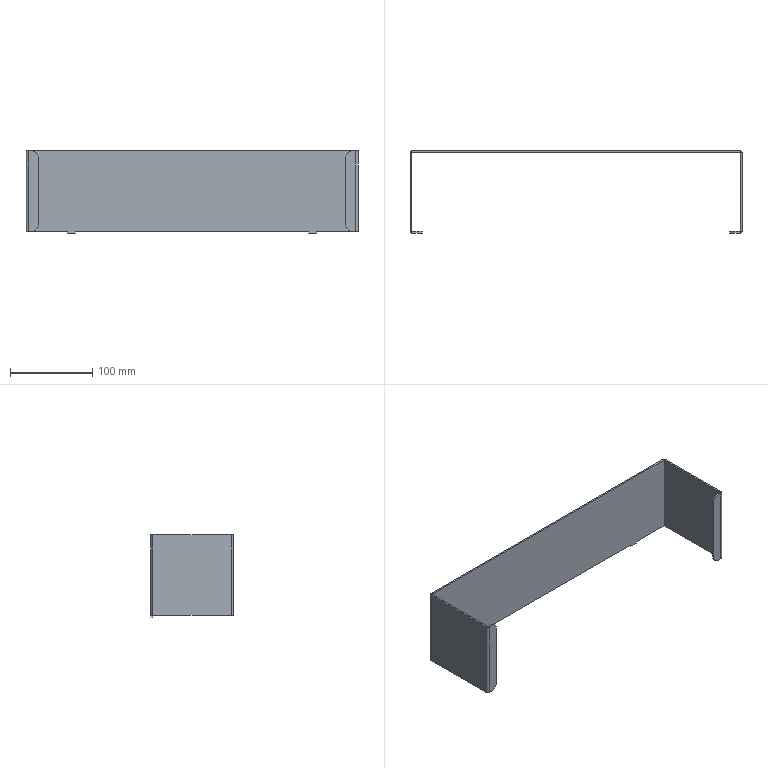Part | STEP file | xzz-001 | 1 solid | 34 faces | box 404 x 100 x 100 mm | volume 122161 mm3 | plane 22 | cylinder 12 | commonest cylinder face diameters 1 x4 5 x4 16 x4
STEP:
#1=CARTESIAN_POINT('',(165.,30.,-2.));
#2=VERTEX_POINT('',#1);
#3=CARTESIAN_POINT('',(175.,30.,-2.));
#4=VERTEX_POINT('',#3);
#5=CARTESIAN_POINT('',(-179.,30.,-2.));
#6=DIRECTION('',(1.,0.,0.));
#7=VECTOR('',#6,1000.);
#8=LINE('',#5,#7);
#9=EDGE_CURVE('',#2,#4,#8,.T.);
#10=ORIENTED_EDGE('',*,*,#9,.T.);
#11=CARTESIAN_POINT('',(175.,30.,0.));
#12=VERTEX_POINT('',#11);
#13=CARTESIAN_POINT('',(175.,30.,98.));
#14=DIRECTION('',(0.,0.,1.));
#15=VECTOR('',#14,1000.);
#16=LINE('',#13,#15);
#17=EDGE_CURVE('',#4,#12,#16,.T.);
#18=ORIENTED_EDGE('',*,*,#17,.T.);
#19=CARTESIAN_POINT('',(222.5,30.,0.));
#20=VERTEX_POINT('',#19);
#21=CARTESIAN_POINT('',(-179.,30.,0.));
#22=DIRECTION('',(1.,0.,0.));
#23=VECTOR('',#22,1000.);
#24=LINE('',#21,#23);
#25=EDGE_CURVE('',#12,#20,#24,.T.);
#26=ORIENTED_EDGE('',*,*,#25,.T.);
#27=CARTESIAN_POINT('',(222.5,30.,98.));
#28=VERTEX_POINT('',#27);
#29=CARTESIAN_POINT('',(222.5,30.,98.));
#30=DIRECTION('',(0.,0.,1.));
#31=VECTOR('',#30,1000.);
#32=LINE('',#29,#31);
#33=EDGE_CURVE('',#20,#28,#32,.T.);
#34=ORIENTED_EDGE('',*,*,#33,.T.);
#35=CARTESIAN_POINT('',(-176.5,30.,98.));
#36=VERTEX_POINT('',#35);
#37=CARTESIAN_POINT('',(-179.,30.,98.));
#38=DIRECTION('',(-1.,0.,0.));
#39=VECTOR('',#38,1000.);
#40=LINE('',#37,#39);
#41=EDGE_CURVE('',#28,#36,#40,.T.);
#42=ORIENTED_EDGE('',*,*,#41,.T.);
#43=CARTESIAN_POINT('',(-176.5,30.,0.));
#44=VERTEX_POINT('',#43);
#45=CARTESIAN_POINT('',(-176.5,30.,98.));
#46=DIRECTION('',(0.,0.,-1.));
#47=VECTOR('',#46,1000.);
#48=LINE('',#45,#47);
#49=EDGE_CURVE('',#36,#44,#48,.T.);
#50=ORIENTED_EDGE('',*,*,#49,.T.);
#51=CARTESIAN_POINT('',(-129.,30.,0.));
#52=VERTEX_POINT('',#51);
#53=CARTESIAN_POINT('',(-179.,30.,0.));
#54=DIRECTION('',(1.,0.,0.));
#55=VECTOR('',#54,1000.);
#56=LINE('',#53,#55);
#57=EDGE_CURVE('',#44,#52,#56,.T.);
#58=ORIENTED_EDGE('',*,*,#57,.T.);
#59=CARTESIAN_POINT('',(-129.,30.,-2.));
#60=VERTEX_POINT('',#59);
#61=CARTESIAN_POINT('',(-129.,30.,98.));
#62=DIRECTION('',(0.,0.,-1.));
#63=VECTOR('',#62,1000.);
#64=LINE('',#61,#63);
#65=EDGE_CURVE('',#52,#60,#64,.T.);
#66=ORIENTED_EDGE('',*,*,#65,.T.);
#67=CARTESIAN_POINT('',(-119.,30.,-2.));
#68=VERTEX_POINT('',#67);
#69=CARTESIAN_POINT('',(-179.,30.,-2.));
#70=DIRECTION('',(1.,0.,0.));
#71=VECTOR('',#70,1000.);
#72=LINE('',#69,#71);
#73=EDGE_CURVE('',#60,#68,#72,.T.);
#74=ORIENTED_EDGE('',*,*,#73,.T.);
#75=CARTESIAN_POINT('',(-119.,30.,0.));
#76=VERTEX_POINT('',#75);
#77=CARTESIAN_POINT('',(-119.,30.,98.));
#78=DIRECTION('',(0.,0.,1.));
#79=VECTOR('',#78,1000.);
#80=LINE('',#77,#79);
#81=EDGE_CURVE('',#68,#76,#80,.T.);
#82=ORIENTED_EDGE('',*,*,#81,.T.);
#83=CARTESIAN_POINT('',(165.,30.,0.));
#84=VERTEX_POINT('',#83);
#85=CARTESIAN_POINT('',(-179.,30.,0.));
#86=DIRECTION('',(1.,0.,0.));
#87=VECTOR('',#86,1000.);
#88=LINE('',#85,#87);
#89=EDGE_CURVE('',#76,#84,#88,.T.);
#90=ORIENTED_EDGE('',*,*,#89,.T.);
#91=CARTESIAN_POINT('',(165.,30.,98.));
#92=DIRECTION('',(0.,0.,-1.));
#93=VECTOR('',#92,1000.);
#94=LINE('',#91,#93);
#95=EDGE_CURVE('',#84,#2,#94,.T.);
#96=ORIENTED_EDGE('',*,*,#95,.T.);
#97=EDGE_LOOP('',(#10,#18,#26,#34,#42,#50,#58,#66,#74,#82,#90,#96));
#98=FACE_OUTER_BOUND('',#97,.T.);
#99=CARTESIAN_POINT('',(-179.,30.,98.));
#100=DIRECTION('',(0.,-1.,0.));
#101=DIRECTION('',(0.,0.,-1.));
#102=AXIS2_PLACEMENT_3D('',#99,#100,#101);
#103=PLANE('',#102);
#104=ADVANCED_FACE('',(#98),#103,.T.);
#105=ORIENTED_EDGE('',*,*,#17,.F.);
#106=CARTESIAN_POINT('',(175.,32.,-2.));
#107=VERTEX_POINT('',#106);
#108=CARTESIAN_POINT('',(175.,32.,-2.));
#109=DIRECTION('',(0.,-1.,0.));
#110=VECTOR('',#109,1000.);
#111=LINE('',#108,#110);
#112=EDGE_CURVE('',#107,#4,#111,.T.);
#113=ORIENTED_EDGE('',*,*,#112,.F.);
#114=CARTESIAN_POINT('',(175.,32.,0.));
#115=VERTEX_POINT('',#114);
#116=CARTESIAN_POINT('',(175.,32.,-2.));
#117=DIRECTION('',(0.,0.,-1.));
#118=VECTOR('',#117,1000.);
#119=LINE('',#116,#118);
#120=EDGE_CURVE('',#115,#107,#119,.T.);
#121=ORIENTED_EDGE('',*,*,#120,.F.);
#122=CARTESIAN_POINT('',(175.,32.,0.));
#123=DIRECTION('',(0.,1.,0.));
#124=VECTOR('',#123,1000.);
#125=LINE('',#122,#124);
#126=EDGE_CURVE('',#12,#115,#125,.T.);
#127=ORIENTED_EDGE('',*,*,#126,.F.);
#128=EDGE_LOOP('',(#105,#113,#121,#127));
#129=FACE_OUTER_BOUND('',#128,.T.);
#130=CARTESIAN_POINT('',(175.,32.,-2.));
#131=DIRECTION('',(-1.,0.,0.));
#132=DIRECTION('',(0.,0.,1.));
#133=AXIS2_PLACEMENT_3D('',#130,#131,#132);
#134=PLANE('',#133);
#135=ADVANCED_FACE('',(#129),#134,.F.);
#136=CARTESIAN_POINT('',(165.,32.,-2.));
#137=VERTEX_POINT('',#136);
#138=CARTESIAN_POINT('',(165.,0.,-2.));
#139=DIRECTION('',(0.,1.,0.));
#140=VECTOR('',#139,1000.);
#141=LINE('',#138,#140);
#142=EDGE_CURVE('',#2,#137,#141,.T.);
#143=ORIENTED_EDGE('',*,*,#142,.T.);
#144=CARTESIAN_POINT('',(0.,32.,-2.));
#145=DIRECTION('',(1.,0.,0.));
#146=VECTOR('',#145,1000.);
#147=LINE('',#144,#146);
#148=EDGE_CURVE('',#137,#107,#147,.T.);
#149=ORIENTED_EDGE('',*,*,#148,.T.);
#150=ORIENTED_EDGE('',*,*,#112,.T.);
#151=ORIENTED_EDGE('',*,*,#9,.F.);
#152=EDGE_LOOP('',(#143,#149,#150,#151));
#153=FACE_OUTER_BOUND('',#152,.T.);
#154=CARTESIAN_POINT('',(0.,0.,-2.));
#155=DIRECTION('',(0.,0.,-1.));
#156=DIRECTION('',(-1.,0.,0.));
#157=AXIS2_PLACEMENT_3D('',#154,#155,#156);
#158=PLANE('',#157);
#159=ADVANCED_FACE('',(#153),#158,.T.);
#160=CARTESIAN_POINT('',(165.,32.,0.));
#161=VERTEX_POINT('',#160);
#162=CARTESIAN_POINT('',(165.,32.,-2.));
#163=DIRECTION('',(0.,0.,1.));
#164=VECTOR('',#163,1000.);
#165=LINE('',#162,#164);
#166=EDGE_CURVE('',#137,#161,#165,.T.);
#167=ORIENTED_EDGE('',*,*,#166,.F.);
#168=ORIENTED_EDGE('',*,*,#142,.F.);
#169=ORIENTED_EDGE('',*,*,#95,.F.);
#170=CARTESIAN_POINT('',(165.,32.,0.));
#171=DIRECTION('',(0.,-1.,0.));
#172=VECTOR('',#171,1000.);
#173=LINE('',#170,#172);
#174=EDGE_CURVE('',#161,#84,#173,.T.);
#175=ORIENTED_EDGE('',*,*,#174,.F.);
#176=EDGE_LOOP('',(#167,#168,#169,#175));
#177=FACE_OUTER_BOUND('',#176,.T.);
#178=CARTESIAN_POINT('',(165.,32.,-2.));
#179=DIRECTION('',(1.,0.,0.));
#180=DIRECTION('',(0.,0.,-1.));
#181=AXIS2_PLACEMENT_3D('',#178,#179,#180);
#182=PLANE('',#181);
#183=ADVANCED_FACE('',(#177),#182,.F.);
#184=CARTESIAN_POINT('',(-119.,32.,0.));
#185=VERTEX_POINT('',#184);
#186=CARTESIAN_POINT('',(223.,32.,0.));
#187=DIRECTION('',(1.,0.,0.));
#188=VECTOR('',#187,1000.);
#189=LINE('',#186,#188);
#190=EDGE_CURVE('',#185,#161,#189,.T.);
#191=ORIENTED_EDGE('',*,*,#190,.T.);
#192=ORIENTED_EDGE('',*,*,#174,.T.);
#193=ORIENTED_EDGE('',*,*,#89,.F.);
#194=CARTESIAN_POINT('',(-119.,29.5,0.));
#195=DIRECTION('',(0.,1.,0.));
#196=VECTOR('',#195,1000.);
#197=LINE('',#194,#196);
#198=EDGE_CURVE('',#76,#185,#197,.T.);
#199=ORIENTED_EDGE('',*,*,#198,.T.);
#200=EDGE_LOOP('',(#191,#192,#193,#199));
#201=FACE_OUTER_BOUND('',#200,.T.);
#202=CARTESIAN_POINT('',(223.,29.5,0.));
#203=DIRECTION('',(0.,0.,-1.));
#204=DIRECTION('',(-1.,0.,0.));
#205=AXIS2_PLACEMENT_3D('',#202,#203,#204);
#206=PLANE('',#205);
#207=ADVANCED_FACE('',(#201),#206,.T.);
#208=ORIENTED_EDGE('',*,*,#81,.F.);
#209=CARTESIAN_POINT('',(-119.,32.,-2.));
#210=VERTEX_POINT('',#209);
#211=CARTESIAN_POINT('',(-119.,32.,-2.));
#212=DIRECTION('',(0.,-1.,0.));
#213=VECTOR('',#212,1000.);
#214=LINE('',#211,#213);
#215=EDGE_CURVE('',#210,#68,#214,.T.);
#216=ORIENTED_EDGE('',*,*,#215,.F.);
#217=CARTESIAN_POINT('',(-119.,32.,-2.));
#218=DIRECTION('',(0.,0.,-1.));
#219=VECTOR('',#218,1000.);
#220=LINE('',#217,#219);
#221=EDGE_CURVE('',#185,#210,#220,.T.);
#222=ORIENTED_EDGE('',*,*,#221,.F.);
#223=ORIENTED_EDGE('',*,*,#198,.F.);
#224=EDGE_LOOP('',(#208,#216,#222,#223));
#225=FACE_OUTER_BOUND('',#224,.T.);
#226=CARTESIAN_POINT('',(-119.,32.,-2.));
#227=DIRECTION('',(-1.,0.,0.));
#228=DIRECTION('',(0.,0.,1.));
#229=AXIS2_PLACEMENT_3D('',#226,#227,#228);
#230=PLANE('',#229);
#231=ADVANCED_FACE('',(#225),#230,.F.);
#232=CARTESIAN_POINT('',(-129.,32.,-2.));
#233=VERTEX_POINT('',#232);
#234=CARTESIAN_POINT('',(-129.,0.,-2.));
#235=DIRECTION('',(0.,1.,0.));
#236=VECTOR('',#235,1000.);
#237=LINE('',#234,#236);
#238=EDGE_CURVE('',#60,#233,#237,.T.);
#239=ORIENTED_EDGE('',*,*,#238,.T.);
#240=CARTESIAN_POINT('',(0.,32.,-2.));
#241=DIRECTION('',(1.,0.,0.));
#242=VECTOR('',#241,1000.);
#243=LINE('',#240,#242);
#244=EDGE_CURVE('',#233,#210,#243,.T.);
#245=ORIENTED_EDGE('',*,*,#244,.T.);
#246=ORIENTED_EDGE('',*,*,#215,.T.);
#247=ORIENTED_EDGE('',*,*,#73,.F.);
#248=EDGE_LOOP('',(#239,#245,#246,#247));
#249=FACE_OUTER_BOUND('',#248,.T.);
#250=CARTESIAN_POINT('',(0.,0.,-2.));
#251=DIRECTION('',(0.,0.,-1.));
#252=DIRECTION('',(-1.,0.,0.));
#253=AXIS2_PLACEMENT_3D('',#250,#251,#252);
#254=PLANE('',#253);
#255=ADVANCED_FACE('',(#249),#254,.T.);
#256=CARTESIAN_POINT('',(-129.,32.,0.));
#257=VERTEX_POINT('',#256);
#258=CARTESIAN_POINT('',(-129.,32.,-2.));
#259=DIRECTION('',(0.,0.,1.));
#260=VECTOR('',#259,1000.);
#261=LINE('',#258,#260);
#262=EDGE_CURVE('',#233,#257,#261,.T.);
#263=ORIENTED_EDGE('',*,*,#262,.F.);
#264=ORIENTED_EDGE('',*,*,#238,.F.);
#265=ORIENTED_EDGE('',*,*,#65,.F.);
#266=CARTESIAN_POINT('',(-129.,32.,0.));
#267=DIRECTION('',(0.,-1.,0.));
#268=VECTOR('',#267,1000.);
#269=LINE('',#266,#268);
#270=EDGE_CURVE('',#257,#52,#269,.T.);
#271=ORIENTED_EDGE('',*,*,#270,.F.);
#272=EDGE_LOOP('',(#263,#264,#265,#271));
#273=FACE_OUTER_BOUND('',#272,.T.);
#274=CARTESIAN_POINT('',(-129.,32.,-2.));
#275=DIRECTION('',(1.,0.,0.));
#276=DIRECTION('',(0.,0.,-1.));
#277=AXIS2_PLACEMENT_3D('',#274,#275,#276);
#278=PLANE('',#277);
#279=ADVANCED_FACE('',(#273),#278,.F.);
#280=ORIENTED_EDGE('',*,*,#57,.F.);
#281=CARTESIAN_POINT('',(-177.,29.5,0.));
#282=VERTEX_POINT('',#281);
#283=CARTESIAN_POINT('',(-176.5,29.5,0.));
#284=DIRECTION('',(0.,0.,1.));
#285=DIRECTION('',(-1.,0.,0.));
#286=AXIS2_PLACEMENT_3D('',#283,#284,#285);
#287=CIRCLE('',#286,0.5);
#288=EDGE_CURVE('',#44,#282,#287,.T.);
#289=ORIENTED_EDGE('',*,*,#288,.T.);
#290=CARTESIAN_POINT('',(-177.,-65.5,0.));
#291=VERTEX_POINT('',#290);
#292=CARTESIAN_POINT('',(-177.,32.,0.));
#293=DIRECTION('',(0.,1.,0.));
#294=VECTOR('',#293,1000.);
#295=LINE('',#292,#294);
#296=EDGE_CURVE('',#291,#282,#295,.T.);
#297=ORIENTED_EDGE('',*,*,#296,.F.);
#298=CARTESIAN_POINT('',(-176.5,-66.,0.));
#299=VERTEX_POINT('',#298);
#300=CARTESIAN_POINT('',(-176.5,-65.5,0.));
#301=DIRECTION('',(0.,0.,1.));
#302=DIRECTION('',(-1.,0.,0.));
#303=AXIS2_PLACEMENT_3D('',#300,#301,#302);
#304=CIRCLE('',#303,0.5);
#305=EDGE_CURVE('',#291,#299,#304,.T.);
#306=ORIENTED_EDGE('',*,*,#305,.T.);
#307=CARTESIAN_POINT('',(-172.,-66.,0.));
#308=VERTEX_POINT('',#307);
#309=CARTESIAN_POINT('',(-179.,-66.,0.));
#310=DIRECTION('',(-1.,0.,0.));
#311=VECTOR('',#310,1000.);
#312=LINE('',#309,#311);
#313=EDGE_CURVE('',#308,#299,#312,.T.);
#314=ORIENTED_EDGE('',*,*,#313,.F.);
#315=CARTESIAN_POINT('',(-172.,-68.,0.));
#316=VERTEX_POINT('',#315);
#317=CARTESIAN_POINT('',(-172.,-65.5,0.));
#318=DIRECTION('',(0.,-1.,0.));
#319=VECTOR('',#318,1000.);
#320=LINE('',#317,#319);
#321=EDGE_CURVE('',#308,#316,#320,.T.);
#322=ORIENTED_EDGE('',*,*,#321,.T.);
#323=CARTESIAN_POINT('',(-176.5,-68.,0.));
#324=VERTEX_POINT('',#323);
#325=CARTESIAN_POINT('',(-177.,-68.,0.));
#326=DIRECTION('',(-1.,0.,0.));
#327=VECTOR('',#326,1000.);
#328=LINE('',#325,#327);
#329=EDGE_CURVE('',#316,#324,#328,.T.);
#330=ORIENTED_EDGE('',*,*,#329,.T.);
#331=CARTESIAN_POINT('',(-179.,-65.5,0.));
#332=VERTEX_POINT('',#331);
#333=CARTESIAN_POINT('',(-176.5,-65.5,0.));
#334=DIRECTION('',(0.,0.,-1.));
#335=DIRECTION('',(-1.,0.,0.));
#336=AXIS2_PLACEMENT_3D('',#333,#334,#335);
#337=CIRCLE('',#336,2.5);
#338=EDGE_CURVE('',#324,#332,#337,.T.);
#339=ORIENTED_EDGE('',*,*,#338,.T.);
#340=CARTESIAN_POINT('',(-179.,29.5,0.));
#341=VERTEX_POINT('',#340);
#342=CARTESIAN_POINT('',(-179.,30.,0.));
#343=DIRECTION('',(0.,1.,0.));
#344=VECTOR('',#343,1000.);
#345=LINE('',#342,#344);
#346=EDGE_CURVE('',#332,#341,#345,.T.);
#347=ORIENTED_EDGE('',*,*,#346,.T.);
#348=CARTESIAN_POINT('',(-176.5,32.,0.));
#349=VERTEX_POINT('',#348);
#350=CARTESIAN_POINT('',(-176.5,29.5,0.));
#351=DIRECTION('',(0.,0.,-1.));
#352=DIRECTION('',(-1.,0.,0.));
#353=AXIS2_PLACEMENT_3D('',#350,#351,#352);
#354=CIRCLE('',#353,2.5);
#355=EDGE_CURVE('',#341,#349,#354,.T.);
#356=ORIENTED_EDGE('',*,*,#355,.T.);
#357=CARTESIAN_POINT('',(223.,32.,0.));
#358=DIRECTION('',(1.,0.,0.));
#359=VECTOR('',#358,1000.);
#360=LINE('',#357,#359);
#361=EDGE_CURVE('',#349,#257,#360,.T.);
#362=ORIENTED_EDGE('',*,*,#361,.T.);
#363=ORIENTED_EDGE('',*,*,#270,.T.);
#364=EDGE_LOOP('',(#280,#289,#297,#306,#314,#322,#330,#339,#347,#356,#362,#363));
#365=FACE_OUTER_BOUND('',#364,.T.);
#366=CARTESIAN_POINT('',(223.,29.5,0.));
#367=DIRECTION('',(0.,0.,-1.));
#368=DIRECTION('',(-1.,0.,0.));
#369=AXIS2_PLACEMENT_3D('',#366,#367,#368);
#370=PLANE('',#369);
#371=ADVANCED_FACE('',(#365),#370,.T.);
#372=ORIENTED_EDGE('',*,*,#49,.F.);
#373=CARTESIAN_POINT('',(-177.,29.5,98.));
#374=VERTEX_POINT('',#373);
#375=CARTESIAN_POINT('',(-176.5,29.5,98.));
#376=DIRECTION('',(0.,0.,-1.));
#377=DIRECTION('',(-1.,0.,0.));
#378=AXIS2_PLACEMENT_3D('',#375,#376,#377);
#379=CIRCLE('',#378,0.5);
#380=EDGE_CURVE('',#374,#36,#379,.T.);
#381=ORIENTED_EDGE('',*,*,#380,.F.);
#382=CARTESIAN_POINT('',(-177.,29.5,98.));
#383=DIRECTION('',(0.,0.,1.));
#384=VECTOR('',#383,1000.);
#385=LINE('',#382,#384);
#386=EDGE_CURVE('',#282,#374,#385,.T.);
#387=ORIENTED_EDGE('',*,*,#386,.F.);
#388=ORIENTED_EDGE('',*,*,#288,.F.);
#389=EDGE_LOOP('',(#372,#381,#387,#388));
#390=FACE_OUTER_BOUND('',#389,.T.);
#391=CARTESIAN_POINT('',(-176.5,29.5,98.));
#392=DIRECTION('',(0.,0.,-1.));
#393=DIRECTION('',(-1.,0.,0.));
#394=AXIS2_PLACEMENT_3D('',#391,#392,#393);
#395=CYLINDRICAL_SURFACE('',#394,0.5);
#396=ADVANCED_FACE('',(#390),#395,.F.);
#397=ORIENTED_EDGE('',*,*,#41,.F.);
#398=CARTESIAN_POINT('',(223.,29.5,98.));
#399=VERTEX_POINT('',#398);
#400=CARTESIAN_POINT('',(222.5,29.5,98.));
#401=DIRECTION('',(0.,0.,-1.));
#402=DIRECTION('',(-1.,0.,0.));
#403=AXIS2_PLACEMENT_3D('',#400,#401,#402);
#404=CIRCLE('',#403,0.5);
#405=EDGE_CURVE('',#28,#399,#404,.T.);
#406=ORIENTED_EDGE('',*,*,#405,.T.);
#407=CARTESIAN_POINT('',(223.,-65.5,98.));
#408=VERTEX_POINT('',#407);
#409=CARTESIAN_POINT('',(223.,32.,98.));
#410=DIRECTION('',(0.,1.,0.));
#411=VECTOR('',#410,1000.);
#412=LINE('',#409,#411);
#413=EDGE_CURVE('',#408,#399,#412,.T.);
#414=ORIENTED_EDGE('',*,*,#413,.F.);
#415=CARTESIAN_POINT('',(222.5,-66.,98.));
#416=VERTEX_POINT('',#415);
#417=CARTESIAN_POINT('',(222.5,-65.5,98.));
#418=DIRECTION('',(0.,0.,-1.));
#419=DIRECTION('',(-1.,0.,0.));
#420=AXIS2_PLACEMENT_3D('',#417,#418,#419);
#421=CIRCLE('',#420,0.5);
#422=EDGE_CURVE('',#408,#416,#421,.T.);
#423=ORIENTED_EDGE('',*,*,#422,.T.);
#424=CARTESIAN_POINT('',(218.,-66.,98.));
#425=VERTEX_POINT('',#424);
#426=CARTESIAN_POINT('',(225.,-66.,98.));
#427=DIRECTION('',(1.,0.,0.));
#428=VECTOR('',#427,1000.);
#429=LINE('',#426,#428);
#430=EDGE_CURVE('',#425,#416,#429,.T.);
#431=ORIENTED_EDGE('',*,*,#430,.F.);
#432=CARTESIAN_POINT('',(218.,-68.,98.));
#433=VERTEX_POINT('',#432);
#434=CARTESIAN_POINT('',(218.,-65.5,98.));
#435=DIRECTION('',(0.,-1.,0.));
#436=VECTOR('',#435,1000.);
#437=LINE('',#434,#436);
#438=EDGE_CURVE('',#425,#433,#437,.T.);
#439=ORIENTED_EDGE('',*,*,#438,.T.);
#440=CARTESIAN_POINT('',(222.5,-68.,98.));
#441=VERTEX_POINT('',#440);
#442=CARTESIAN_POINT('',(223.,-68.,98.));
#443=DIRECTION('',(1.,0.,0.));
#444=VECTOR('',#443,1000.);
#445=LINE('',#442,#444);
#446=EDGE_CURVE('',#433,#441,#445,.T.);
#447=ORIENTED_EDGE('',*,*,#446,.T.);
#448=CARTESIAN_POINT('',(225.,-65.5,98.));
#449=VERTEX_POINT('',#448);
#450=CARTESIAN_POINT('',(222.5,-65.5,98.));
#451=DIRECTION('',(0.,0.,1.));
#452=DIRECTION('',(-1.,0.,0.));
#453=AXIS2_PLACEMENT_3D('',#450,#451,#452);
#454=CIRCLE('',#453,2.5);
#455=EDGE_CURVE('',#441,#449,#454,.T.);
#456=ORIENTED_EDGE('',*,*,#455,.T.);
#457=CARTESIAN_POINT('',(225.,29.5,98.));
#458=VERTEX_POINT('',#457);
#459=CARTESIAN_POINT('',(225.,30.,98.));
#460=DIRECTION('',(0.,1.,0.));
#461=VECTOR('',#460,1000.);
#462=LINE('',#459,#461);
#463=EDGE_CURVE('',#449,#458,#462,.T.);
#464=ORIENTED_EDGE('',*,*,#463,.T.);
#465=CARTESIAN_POINT('',(222.5,32.,98.));
#466=VERTEX_POINT('',#465);
#467=CARTESIAN_POINT('',(222.5,29.5,98.));
#468=DIRECTION('',(0.,0.,1.));
#469=DIRECTION('',(-1.,0.,0.));
#470=AXIS2_PLACEMENT_3D('',#467,#468,#469);
#471=CIRCLE('',#470,2.5);
#472=EDGE_CURVE('',#458,#466,#471,.T.);
#473=ORIENTED_EDGE('',*,*,#472,.T.);
#474=CARTESIAN_POINT('',(-176.5,32.,98.));
#475=VERTEX_POINT('',#474);
#476=CARTESIAN_POINT('',(-177.,32.,98.));
#477=DIRECTION('',(-1.,0.,0.));
#478=VECTOR('',#477,1000.);
#479=LINE('',#476,#478);
#480=EDGE_CURVE('',#466,#475,#479,.T.);
#481=ORIENTED_EDGE('',*,*,#480,.T.);
#482=CARTESIAN_POINT('',(-179.,29.5,98.));
#483=VERTEX_POINT('',#482);
#484=CARTESIAN_POINT('',(-176.5,29.5,98.));
#485=DIRECTION('',(0.,0.,1.));
#486=DIRECTION('',(-1.,0.,0.));
#487=AXIS2_PLACEMENT_3D('',#484,#485,#486);
#488=CIRCLE('',#487,2.5);
#489=EDGE_CURVE('',#475,#483,#488,.T.);
#490=ORIENTED_EDGE('',*,*,#489,.T.);
#491=CARTESIAN_POINT('',(-179.,-65.5,98.));
#492=VERTEX_POINT('',#491);
#493=CARTESIAN_POINT('',(-179.,-66.,98.));
#494=DIRECTION('',(0.,-1.,0.));
#495=VECTOR('',#494,1000.);
#496=LINE('',#493,#495);
#497=EDGE_CURVE('',#483,#492,#496,.T.);
#498=ORIENTED_EDGE('',*,*,#497,.T.);
#499=CARTESIAN_POINT('',(-176.5,-68.,98.));
#500=VERTEX_POINT('',#499);
#501=CARTESIAN_POINT('',(-176.5,-65.5,98.));
#502=DIRECTION('',(0.,0.,1.));
#503=DIRECTION('',(-1.,0.,0.));
#504=AXIS2_PLACEMENT_3D('',#501,#502,#503);
#505=CIRCLE('',#504,2.5);
#506=EDGE_CURVE('',#492,#500,#505,.T.);
#507=ORIENTED_EDGE('',*,*,#506,.T.);
#508=CARTESIAN_POINT('',(-172.,-68.,98.));
#509=VERTEX_POINT('',#508);
#510=CARTESIAN_POINT('',(-176.5,-68.,98.));
#511=DIRECTION('',(1.,0.,0.));
#512=VECTOR('',#511,1000.);
#513=LINE('',#510,#512);
#514=EDGE_CURVE('',#500,#509,#513,.T.);
#515=ORIENTED_EDGE('',*,*,#514,.T.);
#516=CARTESIAN_POINT('',(-172.,-66.,98.));
#517=VERTEX_POINT('',#516);
#518=CARTESIAN_POINT('',(-172.,-66.,98.));
#519=DIRECTION('',(0.,-1.,0.));
#520=VECTOR('',#519,1000.);
#521=LINE('',#518,#520);
#522=EDGE_CURVE('',#517,#509,#521,.T.);
#523=ORIENTED_EDGE('',*,*,#522,.F.);
#524=CARTESIAN_POINT('',(-176.5,-66.,98.));
#525=VERTEX_POINT('',#524);
#526=CARTESIAN_POINT('',(-179.,-66.,98.));
#527=DIRECTION('',(1.,0.,0.));
#528=VECTOR('',#527,1000.);
#529=LINE('',#526,#528);
#530=EDGE_CURVE('',#525,#517,#529,.T.);
#531=ORIENTED_EDGE('',*,*,#530,.F.);
#532=CARTESIAN_POINT('',(-177.,-65.5,98.));
#533=VERTEX_POINT('',#532);
#534=CARTESIAN_POINT('',(-176.5,-65.5,98.));
#535=DIRECTION('',(0.,0.,-1.));
#536=DIRECTION('',(-1.,0.,0.));
#537=AXIS2_PLACEMENT_3D('',#534,#535,#536);
#538=CIRCLE('',#537,0.5);
#539=EDGE_CURVE('',#525,#533,#538,.T.);
#540=ORIENTED_EDGE('',*,*,#539,.T.);
#541=CARTESIAN_POINT('',(-177.,32.,98.));
#542=DIRECTION('',(0.,-1.,0.));
#543=VECTOR('',#542,1000.);
#544=LINE('',#541,#543);
#545=EDGE_CURVE('',#374,#533,#544,.T.);
#546=ORIENTED_EDGE('',*,*,#545,.F.);
#547=ORIENTED_EDGE('',*,*,#380,.T.);
#548=EDGE_LOOP('',(#397,#406,#414,#423,#431,#439,#447,#456,#464,#473,#481,#490,#498,#507,#515,#523,#531,#540,#546,#547));
#549=FACE_OUTER_BOUND('',#548,.T.);
#550=CARTESIAN_POINT('',(-177.,29.5,98.));
#551=DIRECTION('',(0.,0.,1.));
#552=DIRECTION('',(1.,0.,0.));
#553=AXIS2_PLACEMENT_3D('',#550,#551,#552);
#554=PLANE('',#553);
#555=ADVANCED_FACE('',(#549),#554,.T.);
#556=CARTESIAN_POINT('',(223.,29.5,0.));
#557=VERTEX_POINT('',#556);
#558=CARTESIAN_POINT('',(223.,29.5,98.));
#559=DIRECTION('',(0.,0.,-1.));
#560=VECTOR('',#559,1000.);
#561=LINE('',#558,#560);
#562=EDGE_CURVE('',#399,#557,#561,.T.);
#563=ORIENTED_EDGE('',*,*,#562,.F.);
#564=ORIENTED_EDGE('',*,*,#405,.F.);
#565=ORIENTED_EDGE('',*,*,#33,.F.);
#566=CARTESIAN_POINT('',(222.5,29.5,0.));
#567=DIRECTION('',(0.,0.,1.));
#568=DIRECTION('',(-1.,0.,0.));
#569=AXIS2_PLACEMENT_3D('',#566,#567,#568);
#570=CIRCLE('',#569,0.5);
#571=EDGE_CURVE('',#557,#20,#570,.T.);
#572=ORIENTED_EDGE('',*,*,#571,.F.);
#573=EDGE_LOOP('',(#563,#564,#565,#572));
#574=FACE_OUTER_BOUND('',#573,.T.);
#575=CARTESIAN_POINT('',(222.5,29.5,98.));
#576=DIRECTION('',(0.,0.,-1.));
#577=DIRECTION('',(-1.,0.,0.));
#578=AXIS2_PLACEMENT_3D('',#575,#576,#577);
#579=CYLINDRICAL_SURFACE('',#578,0.5);
#580=ADVANCED_FACE('',(#574),#579,.F.);
#581=CARTESIAN_POINT('',(222.5,32.,0.));
#582=VERTEX_POINT('',#581);
#583=CARTESIAN_POINT('',(223.,32.,0.));
#584=DIRECTION('',(1.,0.,0.));
#585=VECTOR('',#584,1000.);
#586=LINE('',#583,#585);
#587=EDGE_CURVE('',#115,#582,#586,.T.);
#588=ORIENTED_EDGE('',*,*,#587,.T.);
#589=CARTESIAN_POINT('',(225.,29.5,0.));
#590=VERTEX_POINT('',#589);
#591=CARTESIAN_POINT('',(222.5,29.5,0.));
#592=DIRECTION('',(0.,0.,-1.));
#593=DIRECTION('',(-1.,0.,0.));
#594=AXIS2_PLACEMENT_3D('',#591,#592,#593);
#595=CIRCLE('',#594,2.5);
#596=EDGE_CURVE('',#582,#590,#595,.T.);
#597=ORIENTED_EDGE('',*,*,#596,.T.);
#598=CARTESIAN_POINT('',(225.,-65.5,0.));
#599=VERTEX_POINT('',#598);
#600=CARTESIAN_POINT('',(225.,-66.,0.));
#601=DIRECTION('',(0.,-1.,0.));
#602=VECTOR('',#601,1000.);
#603=LINE('',#600,#602);
#604=EDGE_CURVE('',#590,#599,#603,.T.);
#605=ORIENTED_EDGE('',*,*,#604,.T.);
#606=CARTESIAN_POINT('',(222.5,-68.,0.));
#607=VERTEX_POINT('',#606);
#608=CARTESIAN_POINT('',(222.5,-65.5,0.));
#609=DIRECTION('',(0.,0.,-1.));
#610=DIRECTION('',(-1.,0.,0.));
#611=AXIS2_PLACEMENT_3D('',#608,#609,#610);
#612=CIRCLE('',#611,2.5);
#613=EDGE_CURVE('',#599,#607,#612,.T.);
#614=ORIENTED_EDGE('',*,*,#613,.T.);
#615=CARTESIAN_POINT('',(218.,-68.,0.));
#616=VERTEX_POINT('',#615);
#617=CARTESIAN_POINT('',(-176.5,-68.,0.));
#618=DIRECTION('',(1.,0.,0.));
#619=VECTOR('',#618,1000.);
#620=LINE('',#617,#619);
#621=EDGE_CURVE('',#616,#607,#620,.T.);
#622=ORIENTED_EDGE('',*,*,#621,.F.);
#623=CARTESIAN_POINT('',(218.,-66.,0.));
#624=VERTEX_POINT('',#623);
#625=CARTESIAN_POINT('',(218.,-65.5,0.));
#626=DIRECTION('',(0.,-1.,0.));
#627=VECTOR('',#626,1000.);
#628=LINE('',#625,#627);
#629=EDGE_CURVE('',#624,#616,#628,.T.);
#630=ORIENTED_EDGE('',*,*,#629,.F.);
#631=CARTESIAN_POINT('',(222.5,-66.,0.));
#632=VERTEX_POINT('',#631);
#633=CARTESIAN_POINT('',(225.,-66.,0.));
#634=DIRECTION('',(-1.,0.,0.));
#635=VECTOR('',#634,1000.);
#636=LINE('',#633,#635);
#637=EDGE_CURVE('',#632,#624,#636,.T.);
#638=ORIENTED_EDGE('',*,*,#637,.F.);
#639=CARTESIAN_POINT('',(223.,-65.5,0.));
#640=VERTEX_POINT('',#639);
#641=CARTESIAN_POINT('',(222.5,-65.5,0.));
#642=DIRECTION('',(0.,0.,1.));
#643=DIRECTION('',(-1.,0.,0.));
#644=AXIS2_PLACEMENT_3D('',#641,#642,#643);
#645=CIRCLE('',#644,0.5);
#646=EDGE_CURVE('',#632,#640,#645,.T.);
#647=ORIENTED_EDGE('',*,*,#646,.T.);
#648=CARTESIAN_POINT('',(223.,32.,0.));
#649=DIRECTION('',(0.,-1.,0.));
#650=VECTOR('',#649,1000.);
#651=LINE('',#648,#650);
#652=EDGE_CURVE('',#557,#640,#651,.T.);
#653=ORIENTED_EDGE('',*,*,#652,.F.);
#654=ORIENTED_EDGE('',*,*,#571,.T.);
#655=ORIENTED_EDGE('',*,*,#25,.F.);
#656=ORIENTED_EDGE('',*,*,#126,.T.);
#657=EDGE_LOOP('',(#588,#597,#605,#614,#622,#630,#638,#647,#653,#654,#655,#656));
#658=FACE_OUTER_BOUND('',#657,.T.);
#659=CARTESIAN_POINT('',(223.,29.5,0.));
#660=DIRECTION('',(0.,0.,-1.));
#661=DIRECTION('',(-1.,0.,0.));
#662=AXIS2_PLACEMENT_3D('',#659,#660,#661);
#663=PLANE('',#662);
#664=ADVANCED_FACE('',(#658),#663,.T.);
#665=ORIENTED_EDGE('',*,*,#120,.T.);
#666=ORIENTED_EDGE('',*,*,#148,.F.);
#667=ORIENTED_EDGE('',*,*,#166,.T.);
#668=ORIENTED_EDGE('',*,*,#190,.F.);
#669=ORIENTED_EDGE('',*,*,#221,.T.);
#670=ORIENTED_EDGE('',*,*,#244,.F.);
#671=ORIENTED_EDGE('',*,*,#262,.T.);
#672=ORIENTED_EDGE('',*,*,#361,.F.);
#673=CARTESIAN_POINT('',(-176.5,32.,98.));
#674=DIRECTION('',(0.,0.,-1.));
#675=VECTOR('',#674,1000.);
#676=LINE('',#673,#675);
#677=EDGE_CURVE('',#475,#349,#676,.T.);
#678=ORIENTED_EDGE('',*,*,#677,.F.);
#679=ORIENTED_EDGE('',*,*,#480,.F.);
#680=CARTESIAN_POINT('',(222.5,32.,98.));
#681=DIRECTION('',(0.,0.,1.));
#682=VECTOR('',#681,1000.);
#683=LINE('',#680,#682);
#684=EDGE_CURVE('',#582,#466,#683,.T.);
#685=ORIENTED_EDGE('',*,*,#684,.F.);
#686=ORIENTED_EDGE('',*,*,#587,.F.);
#687=EDGE_LOOP('',(#665,#666,#667,#668,#669,#670,#671,#672,#678,#679,#685,#686));
#688=FACE_OUTER_BOUND('',#687,.T.);
#689=CARTESIAN_POINT('',(-179.,32.,98.));
#690=DIRECTION('',(0.,-1.,0.));
#691=DIRECTION('',(0.,0.,-1.));
#692=AXIS2_PLACEMENT_3D('',#689,#690,#691);
#693=PLANE('',#692);
#694=ADVANCED_FACE('',(#688),#693,.F.);
#695=ORIENTED_EDGE('',*,*,#545,.T.);
#696=CARTESIAN_POINT('',(-177.,-65.5,98.));
#697=DIRECTION('',(0.,0.,-1.));
#698=VECTOR('',#697,1000.);
#699=LINE('',#696,#698);
#700=EDGE_CURVE('',#533,#291,#699,.T.);
#701=ORIENTED_EDGE('',*,*,#700,.T.);
#702=ORIENTED_EDGE('',*,*,#296,.T.);
#703=ORIENTED_EDGE('',*,*,#386,.T.);
#704=EDGE_LOOP('',(#695,#701,#702,#703));
#705=FACE_OUTER_BOUND('',#704,.T.);
#706=CARTESIAN_POINT('',(-177.,32.,98.));
#707=DIRECTION('',(1.,0.,0.));
#708=DIRECTION('',(0.,1.,0.));
#709=AXIS2_PLACEMENT_3D('',#706,#707,#708);
#710=PLANE('',#709);
#711=ADVANCED_FACE('',(#705),#710,.T.);
#712=ORIENTED_EDGE('',*,*,#413,.T.);
#713=ORIENTED_EDGE('',*,*,#562,.T.);
#714=ORIENTED_EDGE('',*,*,#652,.T.);
#715=CARTESIAN_POINT('',(223.,-65.5,98.));
#716=DIRECTION('',(0.,0.,1.));
#717=VECTOR('',#716,1000.);
#718=LINE('',#715,#717);
#719=EDGE_CURVE('',#640,#408,#718,.T.);
#720=ORIENTED_EDGE('',*,*,#719,.T.);
#721=EDGE_LOOP('',(#712,#713,#714,#720));
#722=FACE_OUTER_BOUND('',#721,.T.);
#723=CARTESIAN_POINT('',(223.,32.,98.));
#724=DIRECTION('',(-1.,0.,0.));
#725=DIRECTION('',(0.,0.,1.));
#726=AXIS2_PLACEMENT_3D('',#723,#724,#725);
#727=PLANE('',#726);
#728=ADVANCED_FACE('',(#722),#727,.T.);
#729=ORIENTED_EDGE('',*,*,#489,.F.);
#730=ORIENTED_EDGE('',*,*,#677,.T.);
#731=ORIENTED_EDGE('',*,*,#355,.F.);
#732=CARTESIAN_POINT('',(-179.,29.5,98.));
#733=DIRECTION('',(0.,0.,1.));
#734=VECTOR('',#733,1000.);
#735=LINE('',#732,#734);
#736=EDGE_CURVE('',#341,#483,#735,.T.);
#737=ORIENTED_EDGE('',*,*,#736,.T.);
#738=EDGE_LOOP('',(#729,#730,#731,#737));
#739=FACE_OUTER_BOUND('',#738,.T.);
#740=CARTESIAN_POINT('',(-176.5,29.5,98.));
#741=DIRECTION('',(0.,0.,-1.));
#742=DIRECTION('',(-1.,0.,0.));
#743=AXIS2_PLACEMENT_3D('',#740,#741,#742);
#744=CYLINDRICAL_SURFACE('',#743,2.5);
#745=ADVANCED_FACE('',(#739),#744,.T.);
#746=ORIENTED_EDGE('',*,*,#472,.F.);
#747=CARTESIAN_POINT('',(225.,29.5,98.));
#748=DIRECTION('',(0.,0.,-1.));
#749=VECTOR('',#748,1000.);
#750=LINE('',#747,#749);
#751=EDGE_CURVE('',#458,#590,#750,.T.);
#752=ORIENTED_EDGE('',*,*,#751,.T.);
#753=ORIENTED_EDGE('',*,*,#596,.F.);
#754=ORIENTED_EDGE('',*,*,#684,.T.);
#755=EDGE_LOOP('',(#746,#752,#753,#754));
#756=FACE_OUTER_BOUND('',#755,.T.);
#757=CARTESIAN_POINT('',(222.5,29.5,98.));
#758=DIRECTION('',(0.,0.,-1.));
#759=DIRECTION('',(-1.,0.,0.));
#760=AXIS2_PLACEMENT_3D('',#757,#758,#759);
#761=CYLINDRICAL_SURFACE('',#760,2.5);
#762=ADVANCED_FACE('',(#756),#761,.T.);
#763=ORIENTED_EDGE('',*,*,#700,.F.);
#764=ORIENTED_EDGE('',*,*,#539,.F.);
#765=CARTESIAN_POINT('',(-176.5,-66.,98.));
#766=DIRECTION('',(0.,0.,1.));
#767=VECTOR('',#766,1000.);
#768=LINE('',#765,#767);
#769=EDGE_CURVE('',#299,#525,#768,.T.);
#770=ORIENTED_EDGE('',*,*,#769,.F.);
#771=ORIENTED_EDGE('',*,*,#305,.F.);
#772=EDGE_LOOP('',(#763,#764,#770,#771));
#773=FACE_OUTER_BOUND('',#772,.T.);
#774=CARTESIAN_POINT('',(-176.5,-65.5,98.));
#775=DIRECTION('',(0.,0.,-1.));
#776=DIRECTION('',(-1.,0.,0.));
#777=AXIS2_PLACEMENT_3D('',#774,#775,#776);
#778=CYLINDRICAL_SURFACE('',#777,0.5);
#779=ADVANCED_FACE('',(#773),#778,.F.);
#780=CARTESIAN_POINT('',(222.5,-66.,98.));
#781=DIRECTION('',(0.,0.,-1.));
#782=VECTOR('',#781,1000.);
#783=LINE('',#780,#782);
#784=EDGE_CURVE('',#416,#632,#783,.T.);
#785=ORIENTED_EDGE('',*,*,#784,.F.);
#786=ORIENTED_EDGE('',*,*,#422,.F.);
#787=ORIENTED_EDGE('',*,*,#719,.F.);
#788=ORIENTED_EDGE('',*,*,#646,.F.);
#789=EDGE_LOOP('',(#785,#786,#787,#788));
#790=FACE_OUTER_BOUND('',#789,.T.);
#791=CARTESIAN_POINT('',(222.5,-65.5,98.));
#792=DIRECTION('',(0.,0.,-1.));
#793=DIRECTION('',(-1.,0.,0.));
#794=AXIS2_PLACEMENT_3D('',#791,#792,#793);
#795=CYLINDRICAL_SURFACE('',#794,0.5);
#796=ADVANCED_FACE('',(#790),#795,.F.);
#797=CARTESIAN_POINT('',(-179.,-65.5,98.));
#798=DIRECTION('',(0.,0.,-1.));
#799=VECTOR('',#798,1000.);
#800=LINE('',#797,#799);
#801=EDGE_CURVE('',#492,#332,#800,.T.);
#802=ORIENTED_EDGE('',*,*,#801,.F.);
#803=ORIENTED_EDGE('',*,*,#497,.F.);
#804=ORIENTED_EDGE('',*,*,#736,.F.);
#805=ORIENTED_EDGE('',*,*,#346,.F.);
#806=EDGE_LOOP('',(#802,#803,#804,#805));
#807=FACE_OUTER_BOUND('',#806,.T.);
#808=CARTESIAN_POINT('',(-179.,32.,98.));
#809=DIRECTION('',(1.,0.,0.));
#810=DIRECTION('',(0.,1.,0.));
#811=AXIS2_PLACEMENT_3D('',#808,#809,#810);
#812=PLANE('',#811);
#813=ADVANCED_FACE('',(#807),#812,.F.);
#814=ORIENTED_EDGE('',*,*,#751,.F.);
#815=ORIENTED_EDGE('',*,*,#463,.F.);
#816=CARTESIAN_POINT('',(225.,-65.5,98.));
#817=DIRECTION('',(0.,0.,1.));
#818=VECTOR('',#817,1000.);
#819=LINE('',#816,#818);
#820=EDGE_CURVE('',#599,#449,#819,.T.);
#821=ORIENTED_EDGE('',*,*,#820,.F.);
#822=ORIENTED_EDGE('',*,*,#604,.F.);
#823=EDGE_LOOP('',(#814,#815,#821,#822));
#824=FACE_OUTER_BOUND('',#823,.T.);
#825=CARTESIAN_POINT('',(225.,32.,98.));
#826=DIRECTION('',(-1.,0.,0.));
#827=DIRECTION('',(0.,0.,1.));
#828=AXIS2_PLACEMENT_3D('',#825,#826,#827);
#829=PLANE('',#828);
#830=ADVANCED_FACE('',(#824),#829,.F.);
#831=ORIENTED_EDGE('',*,*,#530,.T.);
#832=CARTESIAN_POINT('',(-164.,-66.,90.));
#833=VERTEX_POINT('',#832);
#834=CARTESIAN_POINT('',(-172.,-66.,90.));
#835=DIRECTION('',(0.,1.,0.));
#836=DIRECTION('',(0.,0.,-1.));
#837=AXIS2_PLACEMENT_3D('',#834,#835,#836);
#838=CIRCLE('',#837,8.);
#839=EDGE_CURVE('',#517,#833,#838,.T.);
#840=ORIENTED_EDGE('',*,*,#839,.T.);
#841=CARTESIAN_POINT('',(-164.,-66.,8.));
#842=VERTEX_POINT('',#841);
#843=CARTESIAN_POINT('',(-164.,-66.,98.));
#844=DIRECTION('',(0.,0.,-1.));
#845=VECTOR('',#844,1000.);
#846=LINE('',#843,#845);
#847=EDGE_CURVE('',#833,#842,#846,.T.);
#848=ORIENTED_EDGE('',*,*,#847,.T.);
#849=CARTESIAN_POINT('',(-172.,-66.,8.));
#850=DIRECTION('',(0.,1.,0.));
#851=DIRECTION('',(0.,0.,-1.));
#852=AXIS2_PLACEMENT_3D('',#849,#850,#851);
#853=CIRCLE('',#852,8.);
#854=EDGE_CURVE('',#842,#308,#853,.T.);
#855=ORIENTED_EDGE('',*,*,#854,.T.);
#856=ORIENTED_EDGE('',*,*,#313,.T.);
#857=ORIENTED_EDGE('',*,*,#769,.T.);
#858=EDGE_LOOP('',(#831,#840,#848,#855,#856,#857));
#859=FACE_OUTER_BOUND('',#858,.T.);
#860=CARTESIAN_POINT('',(-179.,-66.,98.));
#861=DIRECTION('',(0.,1.,0.));
#862=DIRECTION('',(0.,0.,1.));
#863=AXIS2_PLACEMENT_3D('',#860,#861,#862);
#864=PLANE('',#863);
#865=ADVANCED_FACE('',(#859),#864,.T.);
#866=ORIENTED_EDGE('',*,*,#430,.T.);
#867=ORIENTED_EDGE('',*,*,#784,.T.);
#868=ORIENTED_EDGE('',*,*,#637,.T.);
#869=CARTESIAN_POINT('',(210.,-66.,8.));
#870=VERTEX_POINT('',#869);
#871=CARTESIAN_POINT('',(218.,-66.,8.));
#872=DIRECTION('',(0.,1.,0.));
#873=DIRECTION('',(0.,0.,-1.));
#874=AXIS2_PLACEMENT_3D('',#871,#872,#873);
#875=CIRCLE('',#874,8.);
#876=EDGE_CURVE('',#624,#870,#875,.T.);
#877=ORIENTED_EDGE('',*,*,#876,.T.);
#878=CARTESIAN_POINT('',(210.,-66.,90.));
#879=VERTEX_POINT('',#878);
#880=CARTESIAN_POINT('',(210.,-66.,98.));
#881=DIRECTION('',(0.,0.,1.));
#882=VECTOR('',#881,1000.);
#883=LINE('',#880,#882);
#884=EDGE_CURVE('',#870,#879,#883,.T.);
#885=ORIENTED_EDGE('',*,*,#884,.T.);
#886=CARTESIAN_POINT('',(218.,-66.,90.));
#887=DIRECTION('',(0.,1.,0.));
#888=DIRECTION('',(0.,0.,1.));
#889=AXIS2_PLACEMENT_3D('',#886,#887,#888);
#890=CIRCLE('',#889,8.);
#891=EDGE_CURVE('',#879,#425,#890,.T.);
#892=ORIENTED_EDGE('',*,*,#891,.T.);
#893=EDGE_LOOP('',(#866,#867,#868,#877,#885,#892));
#894=FACE_OUTER_BOUND('',#893,.T.);
#895=CARTESIAN_POINT('',(225.,-66.,98.));
#896=DIRECTION('',(0.,1.,0.));
#897=DIRECTION('',(-1.,0.,0.));
#898=AXIS2_PLACEMENT_3D('',#895,#896,#897);
#899=PLANE('',#898);
#900=ADVANCED_FACE('',(#894),#899,.T.);
#901=ORIENTED_EDGE('',*,*,#506,.F.);
#902=ORIENTED_EDGE('',*,*,#801,.T.);
#903=ORIENTED_EDGE('',*,*,#338,.F.);
#904=CARTESIAN_POINT('',(-176.5,-68.,98.));
#905=DIRECTION('',(0.,0.,1.));
#906=VECTOR('',#905,1000.);
#907=LINE('',#904,#906);
#908=EDGE_CURVE('',#324,#500,#907,.T.);
#909=ORIENTED_EDGE('',*,*,#908,.T.);
#910=EDGE_LOOP('',(#901,#902,#903,#909));
#911=FACE_OUTER_BOUND('',#910,.T.);
#912=CARTESIAN_POINT('',(-176.5,-65.5,98.));
#913=DIRECTION('',(0.,0.,-1.));
#914=DIRECTION('',(-1.,0.,0.));
#915=AXIS2_PLACEMENT_3D('',#912,#913,#914);
#916=CYLINDRICAL_SURFACE('',#915,2.5);
#917=ADVANCED_FACE('',(#911),#916,.T.);
#918=ORIENTED_EDGE('',*,*,#455,.F.);
#919=CARTESIAN_POINT('',(222.5,-68.,98.));
#920=DIRECTION('',(0.,0.,-1.));
#921=VECTOR('',#920,1000.);
#922=LINE('',#919,#921);
#923=EDGE_CURVE('',#441,#607,#922,.T.);
#924=ORIENTED_EDGE('',*,*,#923,.T.);
#925=ORIENTED_EDGE('',*,*,#613,.F.);
#926=ORIENTED_EDGE('',*,*,#820,.T.);
#927=EDGE_LOOP('',(#918,#924,#925,#926));
#928=FACE_OUTER_BOUND('',#927,.T.);
#929=CARTESIAN_POINT('',(222.5,-65.5,98.));
#930=DIRECTION('',(0.,0.,-1.));
#931=DIRECTION('',(-1.,0.,0.));
#932=AXIS2_PLACEMENT_3D('',#929,#930,#931);
#933=CYLINDRICAL_SURFACE('',#932,2.5);
#934=ADVANCED_FACE('',(#928),#933,.T.);
#935=CARTESIAN_POINT('',(-164.,-68.,90.));
#936=VERTEX_POINT('',#935);
#937=CARTESIAN_POINT('',(-172.,-68.,90.));
#938=DIRECTION('',(0.,1.,0.));
#939=DIRECTION('',(0.,0.,-1.));
#940=AXIS2_PLACEMENT_3D('',#937,#938,#939);
#941=CIRCLE('',#940,8.);
#942=EDGE_CURVE('',#509,#936,#941,.T.);
#943=ORIENTED_EDGE('',*,*,#942,.T.);
#944=CARTESIAN_POINT('',(-164.,-66.,90.));
#945=DIRECTION('',(0.,1.,0.));
#946=VECTOR('',#945,1000.);
#947=LINE('',#944,#946);
#948=EDGE_CURVE('',#936,#833,#947,.T.);
#949=ORIENTED_EDGE('',*,*,#948,.T.);
#950=ORIENTED_EDGE('',*,*,#839,.F.);
#951=ORIENTED_EDGE('',*,*,#522,.T.);
#952=EDGE_LOOP('',(#943,#949,#950,#951));
#953=FACE_OUTER_BOUND('',#952,.T.);
#954=CARTESIAN_POINT('',(-172.,-66.,90.));
#955=DIRECTION('',(0.,-1.,0.));
#956=DIRECTION('',(0.,0.,-1.));
#957=AXIS2_PLACEMENT_3D('',#954,#955,#956);
#958=CYLINDRICAL_SURFACE('',#957,8.);
#959=ADVANCED_FACE('',(#953),#958,.T.);
#960=CARTESIAN_POINT('',(-164.,-68.,8.));
#961=VERTEX_POINT('',#960);
#962=CARTESIAN_POINT('',(-172.,-68.,8.));
#963=DIRECTION('',(0.,1.,0.));
#964=DIRECTION('',(0.,0.,-1.));
#965=AXIS2_PLACEMENT_3D('',#962,#963,#964);
#966=CIRCLE('',#965,8.);
#967=EDGE_CURVE('',#961,#316,#966,.T.);
#968=ORIENTED_EDGE('',*,*,#967,.T.);
#969=ORIENTED_EDGE('',*,*,#321,.F.);
#970=ORIENTED_EDGE('',*,*,#854,.F.);
#971=CARTESIAN_POINT('',(-164.,-65.5,8.));
#972=DIRECTION('',(0.,-1.,0.));
#973=VECTOR('',#972,1000.);
#974=LINE('',#971,#973);
#975=EDGE_CURVE('',#842,#961,#974,.T.);
#976=ORIENTED_EDGE('',*,*,#975,.T.);
#977=EDGE_LOOP('',(#968,#969,#970,#976));
#978=FACE_OUTER_BOUND('',#977,.T.);
#979=CARTESIAN_POINT('',(-172.,-65.5,8.));
#980=DIRECTION('',(0.,-1.,0.));
#981=DIRECTION('',(0.,0.,-1.));
#982=AXIS2_PLACEMENT_3D('',#979,#980,#981);
#983=CYLINDRICAL_SURFACE('',#982,8.);
#984=ADVANCED_FACE('',(#978),#983,.T.);
#985=ORIENTED_EDGE('',*,*,#847,.F.);
#986=ORIENTED_EDGE('',*,*,#948,.F.);
#987=CARTESIAN_POINT('',(-164.,-68.,98.));
#988=DIRECTION('',(0.,0.,-1.));
#989=VECTOR('',#988,1000.);
#990=LINE('',#987,#989);
#991=EDGE_CURVE('',#936,#961,#990,.T.);
#992=ORIENTED_EDGE('',*,*,#991,.T.);
#993=ORIENTED_EDGE('',*,*,#975,.F.);
#994=EDGE_LOOP('',(#985,#986,#992,#993));
#995=FACE_OUTER_BOUND('',#994,.T.);
#996=CARTESIAN_POINT('',(-164.,-66.,98.));
#997=DIRECTION('',(1.,0.,0.));
#998=DIRECTION('',(0.,0.,-1.));
#999=AXIS2_PLACEMENT_3D('',#996,#997,#998);
#1000=PLANE('',#999);
#1001=ADVANCED_FACE('',(#995),#1000,.T.);
#1002=ORIENTED_EDGE('',*,*,#891,.F.);
#1003=CARTESIAN_POINT('',(210.,-68.,90.));
#1004=VERTEX_POINT('',#1003);
#1005=CARTESIAN_POINT('',(210.,-68.,90.));
#1006=DIRECTION('',(0.,-1.,0.));
#1007=VECTOR('',#1006,1000.);
#1008=LINE('',#1005,#1007);
#1009=EDGE_CURVE('',#879,#1004,#1008,.T.);
#1010=ORIENTED_EDGE('',*,*,#1009,.T.);
#1011=CARTESIAN_POINT('',(218.,-68.,90.));
#1012=DIRECTION('',(0.,1.,0.));
#1013=DIRECTION('',(0.,0.,1.));
#1014=AXIS2_PLACEMENT_3D('',#1011,#1012,#1013);
#1015=CIRCLE('',#1014,8.);
#1016=EDGE_CURVE('',#1004,#433,#1015,.T.);
#1017=ORIENTED_EDGE('',*,*,#1016,.T.);
#1018=ORIENTED_EDGE('',*,*,#438,.F.);
#1019=EDGE_LOOP('',(#1002,#1010,#1017,#1018));
#1020=FACE_OUTER_BOUND('',#1019,.T.);
#1021=CARTESIAN_POINT('',(218.,-68.,90.));
#1022=DIRECTION('',(0.,1.,0.));
#1023=DIRECTION('',(0.,0.,1.));
#1024=AXIS2_PLACEMENT_3D('',#1021,#1022,#1023);
#1025=CYLINDRICAL_SURFACE('',#1024,8.);
#1026=ADVANCED_FACE('',(#1020),#1025,.T.);
#1027=CARTESIAN_POINT('',(210.,-68.,8.));
#1028=VERTEX_POINT('',#1027);
#1029=CARTESIAN_POINT('',(210.,-68.,98.));
#1030=DIRECTION('',(0.,0.,1.));
#1031=VECTOR('',#1030,1000.);
#1032=LINE('',#1029,#1031);
#1033=EDGE_CURVE('',#1028,#1004,#1032,.T.);
#1034=ORIENTED_EDGE('',*,*,#1033,.T.);
#1035=ORIENTED_EDGE('',*,*,#1009,.F.);
#1036=ORIENTED_EDGE('',*,*,#884,.F.);
#1037=CARTESIAN_POINT('',(210.,-68.,8.));
#1038=DIRECTION('',(0.,-1.,0.));
#1039=VECTOR('',#1038,1000.);
#1040=LINE('',#1037,#1039);
#1041=EDGE_CURVE('',#870,#1028,#1040,.T.);
#1042=ORIENTED_EDGE('',*,*,#1041,.T.);
#1043=EDGE_LOOP('',(#1034,#1035,#1036,#1042));
#1044=FACE_OUTER_BOUND('',#1043,.T.);
#1045=CARTESIAN_POINT('',(210.,-68.,98.));
#1046=DIRECTION('',(-1.,0.,0.));
#1047=DIRECTION('',(0.,0.,1.));
#1048=AXIS2_PLACEMENT_3D('',#1045,#1046,#1047);
#1049=PLANE('',#1048);
#1050=ADVANCED_FACE('',(#1044),#1049,.T.);
#1051=ORIENTED_EDGE('',*,*,#876,.F.);
#1052=ORIENTED_EDGE('',*,*,#629,.T.);
#1053=CARTESIAN_POINT('',(218.,-68.,8.));
#1054=DIRECTION('',(0.,1.,0.));
#1055=DIRECTION('',(0.,0.,-1.));
#1056=AXIS2_PLACEMENT_3D('',#1053,#1054,#1055);
#1057=CIRCLE('',#1056,8.);
#1058=EDGE_CURVE('',#616,#1028,#1057,.T.);
#1059=ORIENTED_EDGE('',*,*,#1058,.T.);
#1060=ORIENTED_EDGE('',*,*,#1041,.F.);
#1061=EDGE_LOOP('',(#1051,#1052,#1059,#1060));
#1062=FACE_OUTER_BOUND('',#1061,.T.);
#1063=CARTESIAN_POINT('',(218.,-65.5,8.));
#1064=DIRECTION('',(0.,-1.,0.));
#1065=DIRECTION('',(0.,0.,-1.));
#1066=AXIS2_PLACEMENT_3D('',#1063,#1064,#1065);
#1067=CYLINDRICAL_SURFACE('',#1066,8.);
#1068=ADVANCED_FACE('',(#1062),#1067,.T.);
#1069=ORIENTED_EDGE('',*,*,#967,.F.);
#1070=ORIENTED_EDGE('',*,*,#991,.F.);
#1071=ORIENTED_EDGE('',*,*,#942,.F.);
#1072=ORIENTED_EDGE('',*,*,#514,.F.);
#1073=ORIENTED_EDGE('',*,*,#908,.F.);
#1074=ORIENTED_EDGE('',*,*,#329,.F.);
#1075=EDGE_LOOP('',(#1069,#1070,#1071,#1072,#1073,#1074));
#1076=FACE_OUTER_BOUND('',#1075,.T.);
#1077=CARTESIAN_POINT('',(-179.,-68.,98.));
#1078=DIRECTION('',(0.,1.,0.));
#1079=DIRECTION('',(0.,0.,1.));
#1080=AXIS2_PLACEMENT_3D('',#1077,#1078,#1079);
#1081=PLANE('',#1080);
#1082=ADVANCED_FACE('',(#1076),#1081,.F.);
#1083=ORIENTED_EDGE('',*,*,#1058,.F.);
#1084=ORIENTED_EDGE('',*,*,#621,.T.);
#1085=ORIENTED_EDGE('',*,*,#923,.F.);
#1086=ORIENTED_EDGE('',*,*,#446,.F.);
#1087=ORIENTED_EDGE('',*,*,#1016,.F.);
#1088=ORIENTED_EDGE('',*,*,#1033,.F.);
#1089=EDGE_LOOP('',(#1083,#1084,#1085,#1086,#1087,#1088));
#1090=FACE_OUTER_BOUND('',#1089,.T.);
#1091=CARTESIAN_POINT('',(225.,-68.,98.));
#1092=DIRECTION('',(0.,1.,0.));
#1093=DIRECTION('',(-1.,0.,0.));
#1094=AXIS2_PLACEMENT_3D('',#1091,#1092,#1093);
#1095=PLANE('',#1094);
#1096=ADVANCED_FACE('',(#1090),#1095,.F.);
#1097=CLOSED_SHELL('',(#104,#135,#159,#183,#207,#231,#255,#279,#371,#396,#555,#580,#664,#694,#711,#728,#745,#762,#779,#796,#813,#830,#865,#900,#917,#934,#959,#984,#1001,#1026,#1050,#1068,#1082,#1096));
#1098=MANIFOLD_SOLID_BREP('',#1097);
#1099=CARTESIAN_POINT('',(0.,0.,0.));
#1100=DIRECTION('',(0.,0.,1.));
#1101=DIRECTION('',(1.,0.,0.));
#1102=AXIS2_PLACEMENT_3D('',#1099,#1100,#1101);
#1103=(LENGTH_UNIT()NAMED_UNIT(*)SI_UNIT(.MILLI.,.METRE.));
#1104=UNCERTAINTY_MEASURE_WITH_UNIT(LENGTH_MEASURE(0.00001),#1103,'','');
#1105=(NAMED_UNIT(*)PLANE_ANGLE_UNIT()SI_UNIT($,.RADIAN.));
#1106=(NAMED_UNIT(*)SI_UNIT($,.STERADIAN.)SOLID_ANGLE_UNIT());
#1107=(GEOMETRIC_REPRESENTATION_CONTEXT(3)GLOBAL_UNCERTAINTY_ASSIGNED_CONTEXT((#1104))GLOBAL_UNIT_ASSIGNED_CONTEXT((#1103,#1105,#1106))REPRESENTATION_CONTEXT('',''));
#1108=ADVANCED_BREP_SHAPE_REPRESENTATION('',(#1098,#1102),#1107);